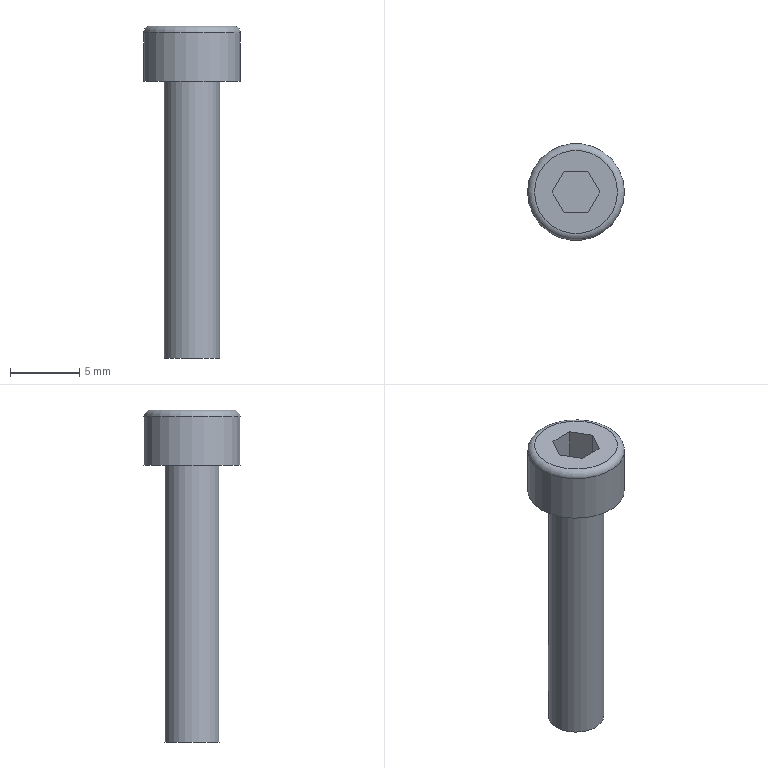Part | STEP file | Tube necking machine_id110_x_t | 1 solid | 13 faces | box 7 x 7 x 24 mm | volume 383.547 mm3 | plane 10 | cylinder 2 | torus 1 | commonest cylinder face diameters 4 x1 7 x1
STEP:
#1=CARTESIAN_POINT('',(0.,0.,0.));
#2=DIRECTION('',(0.,0.,1.));
#3=DIRECTION('',(1.,0.,0.));
#4=AXIS2_PLACEMENT_3D('',#1,#2,#3);
#5=CARTESIAN_POINT('',(-65.,62.5,245.1));
#6=VERTEX_POINT('',#5);
#7=CARTESIAN_POINT('',(-62.,62.5,245.1));
#8=DIRECTION('',(0.,0.,1.));
#9=DIRECTION('',(-1.,0.,0.));
#10=AXIS2_PLACEMENT_3D('',#7,#8,#9);
#11=CIRCLE('',#10,3.);
#12=CARTESIAN_POINT('',(-58.5,62.5,245.1));
#13=DIRECTION('',(0.,0.,-1.));
#14=DIRECTION('',(-1.,0.,0.));
#15=AXIS2_PLACEMENT_3D('',#12,#13,#14);
#16=PLANE('',#15);
#17=CARTESIAN_POINT('',(6.5,0.));
#18=CARTESIAN_POINT('',(6.5,-5.196));
#19=CARTESIAN_POINT('',(2.,-2.598));
#20=CARTESIAN_POINT('',(-2.5,0.));
#21=CARTESIAN_POINT('',(2.,2.598));
#22=CARTESIAN_POINT('',(6.5,5.196));
#23=CARTESIAN_POINT('',(6.5,0.));
#24=(BOUNDED_CURVE()B_SPLINE_CURVE(2,(#17,#18,#19,#20,#21,#22,#23),.UNSPECIFIED.,.T.,.F.)B_SPLINE_CURVE_WITH_KNOTS((1,2,2,2,2,1),(-2.094,0.,2.094,4.189,6.283,8.378),.UNSPECIFIED.)CURVE()GEOMETRIC_REPRESENTATION_ITEM()RATIONAL_B_SPLINE_CURVE((1.,0.5,1.,0.5,1.,0.5,1.))REPRESENTATION_ITEM(''));
#25=(GEOMETRIC_REPRESENTATION_CONTEXT(2)PARAMETRIC_REPRESENTATION_CONTEXT()REPRESENTATION_CONTEXT('',''));
#26=DEFINITIONAL_REPRESENTATION('',(#24),#25);
#27=PCURVE('',#16,#26);
#28=CARTESIAN_POINT('',(-62.,62.5,244.6));
#29=DIRECTION('',(0.,0.,-1.));
#30=DIRECTION('',(-1.,0.,0.));
#31=AXIS2_PLACEMENT_3D('',#28,#29,#30);
#32=TOROIDAL_SURFACE('',#31,3.,0.5);
#33=CARTESIAN_POINT('',(6.283,4.712));
#34=DIRECTION('',(-1.,0.));
#35=VECTOR('',#34,1.);
#36=LINE('',#33,#35);
#37=(GEOMETRIC_REPRESENTATION_CONTEXT(2)PARAMETRIC_REPRESENTATION_CONTEXT()REPRESENTATION_CONTEXT('',''));
#38=DEFINITIONAL_REPRESENTATION('',(#36),#37);
#39=PCURVE('',#32,#38);
#40=SURFACE_CURVE('',#11,(#27,#39),.PCURVE_S1.);
#41=EDGE_CURVE('',#6,#6,#40,.T.);
#42=ORIENTED_EDGE('',*,*,#41,.T.);
#43=EDGE_LOOP('',(#42));
#44=FACE_BOUND('',#43,.T.);
#45=CARTESIAN_POINT('',(-62.866,64.,245.1));
#46=VERTEX_POINT('',#45);
#47=CARTESIAN_POINT('',(-61.134,64.,245.1));
#48=VERTEX_POINT('',#47);
#49=CARTESIAN_POINT('',(-62.866,64.,245.1));
#50=DIRECTION('',(1.,0.,0.));
#51=VECTOR('',#50,1.);
#52=LINE('',#49,#51);
#53=CARTESIAN_POINT('',(4.366,1.5));
#54=DIRECTION('',(-1.,0.));
#55=VECTOR('',#54,1.);
#56=LINE('',#53,#55);
#57=(GEOMETRIC_REPRESENTATION_CONTEXT(2)PARAMETRIC_REPRESENTATION_CONTEXT()REPRESENTATION_CONTEXT('',''));
#58=DEFINITIONAL_REPRESENTATION('',(#56),#57);
#59=PCURVE('',#16,#58);
#60=CARTESIAN_POINT('',(-62.866,64.,242.46));
#61=DIRECTION('',(0.,-1.,0.));
#62=DIRECTION('',(1.,0.,0.));
#63=AXIS2_PLACEMENT_3D('',#60,#61,#62);
#64=PLANE('',#63);
#65=CARTESIAN_POINT('',(0.,2.64));
#66=DIRECTION('',(1.,0.));
#67=VECTOR('',#66,1.);
#68=LINE('',#65,#67);
#69=(GEOMETRIC_REPRESENTATION_CONTEXT(2)PARAMETRIC_REPRESENTATION_CONTEXT()REPRESENTATION_CONTEXT('',''));
#70=DEFINITIONAL_REPRESENTATION('',(#68),#69);
#71=PCURVE('',#64,#70);
#72=SURFACE_CURVE('',#52,(#59,#71),.PCURVE_S1.);
#73=EDGE_CURVE('',#46,#48,#72,.T.);
#74=ORIENTED_EDGE('',*,*,#73,.T.);
#75=CARTESIAN_POINT('',(-60.268,62.5,245.1));
#76=VERTEX_POINT('',#75);
#77=CARTESIAN_POINT('',(-61.134,64.,245.1));
#78=DIRECTION('',(0.5,-0.866,0.));
#79=VECTOR('',#78,1.);
#80=LINE('',#77,#79);
#81=CARTESIAN_POINT('',(2.634,1.5));
#82=DIRECTION('',(-0.5,-0.866));
#83=VECTOR('',#82,1.);
#84=LINE('',#81,#83);
#85=(GEOMETRIC_REPRESENTATION_CONTEXT(2)PARAMETRIC_REPRESENTATION_CONTEXT()REPRESENTATION_CONTEXT('',''));
#86=DEFINITIONAL_REPRESENTATION('',(#84),#85);
#87=PCURVE('',#16,#86);
#88=CARTESIAN_POINT('',(-61.134,64.,242.46));
#89=DIRECTION('',(-0.866,-0.5,0.));
#90=DIRECTION('',(0.5,-0.866,0.));
#91=AXIS2_PLACEMENT_3D('',#88,#89,#90);
#92=PLANE('',#91);
#93=CARTESIAN_POINT('',(0.,2.64));
#94=DIRECTION('',(1.,0.));
#95=VECTOR('',#94,1.);
#96=LINE('',#93,#95);
#97=(GEOMETRIC_REPRESENTATION_CONTEXT(2)PARAMETRIC_REPRESENTATION_CONTEXT()REPRESENTATION_CONTEXT('',''));
#98=DEFINITIONAL_REPRESENTATION('',(#96),#97);
#99=PCURVE('',#92,#98);
#100=SURFACE_CURVE('',#80,(#87,#99),.PCURVE_S1.);
#101=EDGE_CURVE('',#48,#76,#100,.T.);
#102=ORIENTED_EDGE('',*,*,#101,.T.);
#103=CARTESIAN_POINT('',(-61.134,61.,245.1));
#104=VERTEX_POINT('',#103);
#105=CARTESIAN_POINT('',(-60.268,62.5,245.1));
#106=DIRECTION('',(-0.5,-0.866,0.));
#107=VECTOR('',#106,1.);
#108=LINE('',#105,#107);
#109=CARTESIAN_POINT('',(1.768,0.));
#110=DIRECTION('',(0.5,-0.866));
#111=VECTOR('',#110,1.);
#112=LINE('',#109,#111);
#113=(GEOMETRIC_REPRESENTATION_CONTEXT(2)PARAMETRIC_REPRESENTATION_CONTEXT()REPRESENTATION_CONTEXT('',''));
#114=DEFINITIONAL_REPRESENTATION('',(#112),#113);
#115=PCURVE('',#16,#114);
#116=CARTESIAN_POINT('',(-60.268,62.5,242.46));
#117=DIRECTION('',(-0.866,0.5,0.));
#118=DIRECTION('',(-0.5,-0.866,0.));
#119=AXIS2_PLACEMENT_3D('',#116,#117,#118);
#120=PLANE('',#119);
#121=CARTESIAN_POINT('',(0.,2.64));
#122=DIRECTION('',(1.,0.));
#123=VECTOR('',#122,1.);
#124=LINE('',#121,#123);
#125=(GEOMETRIC_REPRESENTATION_CONTEXT(2)PARAMETRIC_REPRESENTATION_CONTEXT()REPRESENTATION_CONTEXT('',''));
#126=DEFINITIONAL_REPRESENTATION('',(#124),#125);
#127=PCURVE('',#120,#126);
#128=SURFACE_CURVE('',#108,(#115,#127),.PCURVE_S1.);
#129=EDGE_CURVE('',#76,#104,#128,.T.);
#130=ORIENTED_EDGE('',*,*,#129,.T.);
#131=CARTESIAN_POINT('',(-62.866,61.,245.1));
#132=VERTEX_POINT('',#131);
#133=CARTESIAN_POINT('',(-61.134,61.,245.1));
#134=DIRECTION('',(-1.,0.,0.));
#135=VECTOR('',#134,1.);
#136=LINE('',#133,#135);
#137=CARTESIAN_POINT('',(2.634,-1.5));
#138=DIRECTION('',(1.,0.));
#139=VECTOR('',#138,1.);
#140=LINE('',#137,#139);
#141=(GEOMETRIC_REPRESENTATION_CONTEXT(2)PARAMETRIC_REPRESENTATION_CONTEXT()REPRESENTATION_CONTEXT('',''));
#142=DEFINITIONAL_REPRESENTATION('',(#140),#141);
#143=PCURVE('',#16,#142);
#144=CARTESIAN_POINT('',(-61.134,61.,242.46));
#145=DIRECTION('',(0.,1.,0.));
#146=DIRECTION('',(-1.,0.,0.));
#147=AXIS2_PLACEMENT_3D('',#144,#145,#146);
#148=PLANE('',#147);
#149=CARTESIAN_POINT('',(0.,2.64));
#150=DIRECTION('',(1.,0.));
#151=VECTOR('',#150,1.);
#152=LINE('',#149,#151);
#153=(GEOMETRIC_REPRESENTATION_CONTEXT(2)PARAMETRIC_REPRESENTATION_CONTEXT()REPRESENTATION_CONTEXT('',''));
#154=DEFINITIONAL_REPRESENTATION('',(#152),#153);
#155=PCURVE('',#148,#154);
#156=SURFACE_CURVE('',#136,(#143,#155),.PCURVE_S1.);
#157=EDGE_CURVE('',#104,#132,#156,.T.);
#158=ORIENTED_EDGE('',*,*,#157,.T.);
#159=CARTESIAN_POINT('',(-63.732,62.5,245.1));
#160=VERTEX_POINT('',#159);
#161=CARTESIAN_POINT('',(-62.866,61.,245.1));
#162=DIRECTION('',(-0.5,0.866,0.));
#163=VECTOR('',#162,1.);
#164=LINE('',#161,#163);
#165=CARTESIAN_POINT('',(4.366,-1.5));
#166=DIRECTION('',(0.5,0.866));
#167=VECTOR('',#166,1.);
#168=LINE('',#165,#167);
#169=(GEOMETRIC_REPRESENTATION_CONTEXT(2)PARAMETRIC_REPRESENTATION_CONTEXT()REPRESENTATION_CONTEXT('',''));
#170=DEFINITIONAL_REPRESENTATION('',(#168),#169);
#171=PCURVE('',#16,#170);
#172=CARTESIAN_POINT('',(-62.866,61.,242.46));
#173=DIRECTION('',(0.866,0.5,0.));
#174=DIRECTION('',(-0.5,0.866,0.));
#175=AXIS2_PLACEMENT_3D('',#172,#173,#174);
#176=PLANE('',#175);
#177=CARTESIAN_POINT('',(0.,2.64));
#178=DIRECTION('',(1.,0.));
#179=VECTOR('',#178,1.);
#180=LINE('',#177,#179);
#181=(GEOMETRIC_REPRESENTATION_CONTEXT(2)PARAMETRIC_REPRESENTATION_CONTEXT()REPRESENTATION_CONTEXT('',''));
#182=DEFINITIONAL_REPRESENTATION('',(#180),#181);
#183=PCURVE('',#176,#182);
#184=SURFACE_CURVE('',#164,(#171,#183),.PCURVE_S1.);
#185=EDGE_CURVE('',#132,#160,#184,.T.);
#186=ORIENTED_EDGE('',*,*,#185,.T.);
#187=CARTESIAN_POINT('',(-63.732,62.5,245.1));
#188=DIRECTION('',(0.5,0.866,0.));
#189=VECTOR('',#188,1.);
#190=LINE('',#187,#189);
#191=CARTESIAN_POINT('',(5.232,0.));
#192=DIRECTION('',(-0.5,0.866));
#193=VECTOR('',#192,1.);
#194=LINE('',#191,#193);
#195=(GEOMETRIC_REPRESENTATION_CONTEXT(2)PARAMETRIC_REPRESENTATION_CONTEXT()REPRESENTATION_CONTEXT('',''));
#196=DEFINITIONAL_REPRESENTATION('',(#194),#195);
#197=PCURVE('',#16,#196);
#198=CARTESIAN_POINT('',(-63.732,62.5,242.46));
#199=DIRECTION('',(0.866,-0.5,0.));
#200=DIRECTION('',(0.5,0.866,0.));
#201=AXIS2_PLACEMENT_3D('',#198,#199,#200);
#202=PLANE('',#201);
#203=CARTESIAN_POINT('',(0.,2.64));
#204=DIRECTION('',(1.,0.));
#205=VECTOR('',#204,1.);
#206=LINE('',#203,#205);
#207=(GEOMETRIC_REPRESENTATION_CONTEXT(2)PARAMETRIC_REPRESENTATION_CONTEXT()REPRESENTATION_CONTEXT('',''));
#208=DEFINITIONAL_REPRESENTATION('',(#206),#207);
#209=PCURVE('',#202,#208);
#210=SURFACE_CURVE('',#190,(#197,#209),.PCURVE_S1.);
#211=EDGE_CURVE('',#160,#46,#210,.T.);
#212=ORIENTED_EDGE('',*,*,#211,.T.);
#213=EDGE_LOOP('',(#74,#102,#130,#158,#186,#212));
#214=FACE_BOUND('',#213,.T.);
#215=ADVANCED_FACE('',(#44,#214),#16,.F.);
#216=CARTESIAN_POINT('',(-65.5,62.5,244.6));
#217=VERTEX_POINT('',#216);
#218=CARTESIAN_POINT('',(-58.5,62.5,244.6));
#219=VERTEX_POINT('',#218);
#220=CARTESIAN_POINT('',(-62.,62.5,244.6));
#221=DIRECTION('',(0.,0.,-1.));
#222=DIRECTION('',(-1.,0.,0.));
#223=AXIS2_PLACEMENT_3D('',#220,#221,#222);
#224=CIRCLE('',#223,3.5);
#225=CARTESIAN_POINT('',(-62.,62.5,242.2));
#226=DIRECTION('',(0.,0.,1.));
#227=DIRECTION('',(1.,0.,0.));
#228=AXIS2_PLACEMENT_3D('',#225,#226,#227);
#229=CYLINDRICAL_SURFACE('',#228,3.5);
#230=CARTESIAN_POINT('',(3.142,2.4));
#231=DIRECTION('',(-1.,0.));
#232=VECTOR('',#231,1.);
#233=LINE('',#230,#232);
#234=(GEOMETRIC_REPRESENTATION_CONTEXT(2)PARAMETRIC_REPRESENTATION_CONTEXT()REPRESENTATION_CONTEXT('',''));
#235=DEFINITIONAL_REPRESENTATION('',(#233),#234);
#236=PCURVE('',#229,#235);
#237=CARTESIAN_POINT('',(0.,6.283));
#238=DIRECTION('',(1.,0.));
#239=VECTOR('',#238,1.);
#240=LINE('',#237,#239);
#241=(GEOMETRIC_REPRESENTATION_CONTEXT(2)PARAMETRIC_REPRESENTATION_CONTEXT()REPRESENTATION_CONTEXT('',''));
#242=DEFINITIONAL_REPRESENTATION('',(#240),#241);
#243=PCURVE('',#32,#242);
#244=SURFACE_CURVE('',#224,(#236,#243),.PCURVE_S1.);
#245=EDGE_CURVE('',#217,#219,#244,.T.);
#246=ORIENTED_EDGE('',*,*,#245,.T.);
#247=CARTESIAN_POINT('',(-58.5,62.5,241.1));
#248=VERTEX_POINT('',#247);
#249=CARTESIAN_POINT('',(-58.5,62.5,241.1));
#250=CARTESIAN_POINT('',(-58.5,62.5,244.6));
#251=B_SPLINE_CURVE_WITH_KNOTS('',1,(#249,#250),.UNSPECIFIED.,.F.,.F.,(2,2),(-1.1,2.4),.PIECEWISE_BEZIER_KNOTS.);
#252=CARTESIAN_POINT('',(0.,0.));
#253=DIRECTION('',(0.,1.));
#254=VECTOR('',#253,1.);
#255=LINE('',#252,#254);
#256=(GEOMETRIC_REPRESENTATION_CONTEXT(2)PARAMETRIC_REPRESENTATION_CONTEXT()REPRESENTATION_CONTEXT('',''));
#257=DEFINITIONAL_REPRESENTATION('',(#255),#256);
#258=PCURVE('',#229,#257);
#259=CARTESIAN_POINT('',(6.283,0.));
#260=DIRECTION('',(0.,1.));
#261=VECTOR('',#260,1.);
#262=LINE('',#259,#261);
#263=(GEOMETRIC_REPRESENTATION_CONTEXT(2)PARAMETRIC_REPRESENTATION_CONTEXT()REPRESENTATION_CONTEXT('',''));
#264=DEFINITIONAL_REPRESENTATION('',(#262),#263);
#265=PCURVE('',#229,#264);
#266=SEAM_CURVE('',#251,(#258,#265),.PCURVE_S1.);
#267=EDGE_CURVE('',#248,#219,#266,.T.);
#268=ORIENTED_EDGE('',*,*,#267,.F.);
#269=CARTESIAN_POINT('',(-62.,62.5,241.1));
#270=DIRECTION('',(0.,0.,1.));
#271=DIRECTION('',(1.,0.,0.));
#272=AXIS2_PLACEMENT_3D('',#269,#270,#271);
#273=CIRCLE('',#272,3.5);
#274=CARTESIAN_POINT('',(0.,-1.1));
#275=DIRECTION('',(1.,0.));
#276=VECTOR('',#275,1.);
#277=LINE('',#274,#276);
#278=(GEOMETRIC_REPRESENTATION_CONTEXT(2)PARAMETRIC_REPRESENTATION_CONTEXT()REPRESENTATION_CONTEXT('',''));
#279=DEFINITIONAL_REPRESENTATION('',(#277),#278);
#280=PCURVE('',#229,#279);
#281=CARTESIAN_POINT('',(-60.,62.5,241.1));
#282=DIRECTION('',(0.,0.,1.));
#283=DIRECTION('',(1.,0.,0.));
#284=AXIS2_PLACEMENT_3D('',#281,#282,#283);
#285=PLANE('',#284);
#286=CARTESIAN_POINT('',(-2.,0.));
#287=DIRECTION('',(1.,0.));
#288=AXIS2_PLACEMENT_2D('',#286,#287);
#289=CIRCLE('',#288,3.5);
#290=(GEOMETRIC_REPRESENTATION_CONTEXT(2)PARAMETRIC_REPRESENTATION_CONTEXT()REPRESENTATION_CONTEXT('',''));
#291=DEFINITIONAL_REPRESENTATION('',(#289),#290);
#292=PCURVE('',#285,#291);
#293=SURFACE_CURVE('',#273,(#280,#292),.PCURVE_S1.);
#294=EDGE_CURVE('',#248,#248,#293,.T.);
#295=ORIENTED_EDGE('',*,*,#294,.T.);
#296=ORIENTED_EDGE('',*,*,#267,.T.);
#297=CARTESIAN_POINT('',(-62.,62.5,244.6));
#298=DIRECTION('',(0.,0.,-1.));
#299=DIRECTION('',(-1.,0.,0.));
#300=AXIS2_PLACEMENT_3D('',#297,#298,#299);
#301=CIRCLE('',#300,3.5);
#302=CARTESIAN_POINT('',(9.425,2.4));
#303=DIRECTION('',(-1.,0.));
#304=VECTOR('',#303,1.);
#305=LINE('',#302,#304);
#306=(GEOMETRIC_REPRESENTATION_CONTEXT(2)PARAMETRIC_REPRESENTATION_CONTEXT()REPRESENTATION_CONTEXT('',''));
#307=DEFINITIONAL_REPRESENTATION('',(#305),#306);
#308=PCURVE('',#229,#307);
#309=CARTESIAN_POINT('',(0.,6.283));
#310=DIRECTION('',(1.,0.));
#311=VECTOR('',#310,1.);
#312=LINE('',#309,#311);
#313=(GEOMETRIC_REPRESENTATION_CONTEXT(2)PARAMETRIC_REPRESENTATION_CONTEXT()REPRESENTATION_CONTEXT('',''));
#314=DEFINITIONAL_REPRESENTATION('',(#312),#313);
#315=PCURVE('',#32,#314);
#316=SURFACE_CURVE('',#301,(#308,#315),.PCURVE_S1.);
#317=EDGE_CURVE('',#219,#217,#316,.T.);
#318=ORIENTED_EDGE('',*,*,#317,.T.);
#319=EDGE_LOOP('',(#246,#268,#295,#296,#318));
#320=FACE_BOUND('',#319,.T.);
#321=ADVANCED_FACE('',(#320),#229,.T.);
#322=ORIENTED_EDGE('',*,*,#294,.F.);
#323=EDGE_LOOP('',(#322));
#324=FACE_BOUND('',#323,.T.);
#325=CARTESIAN_POINT('',(-60.,62.5,241.1));
#326=VERTEX_POINT('',#325);
#327=CARTESIAN_POINT('',(-62.,62.5,241.1));
#328=DIRECTION('',(0.,0.,1.));
#329=DIRECTION('',(1.,0.,0.));
#330=AXIS2_PLACEMENT_3D('',#327,#328,#329);
#331=CIRCLE('',#330,2.);
#332=CARTESIAN_POINT('',(-2.,0.));
#333=DIRECTION('',(1.,0.));
#334=AXIS2_PLACEMENT_2D('',#332,#333);
#335=CIRCLE('',#334,2.);
#336=(GEOMETRIC_REPRESENTATION_CONTEXT(2)PARAMETRIC_REPRESENTATION_CONTEXT()REPRESENTATION_CONTEXT('',''));
#337=DEFINITIONAL_REPRESENTATION('',(#335),#336);
#338=PCURVE('',#285,#337);
#339=CARTESIAN_POINT('',(-62.,62.5,242.2));
#340=DIRECTION('',(0.,0.,1.));
#341=DIRECTION('',(1.,0.,0.));
#342=AXIS2_PLACEMENT_3D('',#339,#340,#341);
#343=CYLINDRICAL_SURFACE('',#342,2.);
#344=CARTESIAN_POINT('',(0.,-1.1));
#345=DIRECTION('',(1.,0.));
#346=VECTOR('',#345,1.);
#347=LINE('',#344,#346);
#348=(GEOMETRIC_REPRESENTATION_CONTEXT(2)PARAMETRIC_REPRESENTATION_CONTEXT()REPRESENTATION_CONTEXT('',''));
#349=DEFINITIONAL_REPRESENTATION('',(#347),#348);
#350=PCURVE('',#343,#349);
#351=SURFACE_CURVE('',#331,(#338,#350),.PCURVE_S1.);
#352=EDGE_CURVE('',#326,#326,#351,.T.);
#353=ORIENTED_EDGE('',*,*,#352,.T.);
#354=EDGE_LOOP('',(#353));
#355=FACE_BOUND('',#354,.T.);
#356=ADVANCED_FACE('',(#324,#355),#285,.F.);
#357=ORIENTED_EDGE('',*,*,#352,.F.);
#358=CARTESIAN_POINT('',(-60.,62.5,221.1));
#359=VERTEX_POINT('',#358);
#360=CARTESIAN_POINT('',(-60.,62.5,221.1));
#361=CARTESIAN_POINT('',(-60.,62.5,241.1));
#362=B_SPLINE_CURVE_WITH_KNOTS('',1,(#360,#361),.UNSPECIFIED.,.F.,.F.,(2,2),(-21.1,-1.1),.PIECEWISE_BEZIER_KNOTS.);
#363=CARTESIAN_POINT('',(0.,0.));
#364=DIRECTION('',(0.,1.));
#365=VECTOR('',#364,1.);
#366=LINE('',#363,#365);
#367=(GEOMETRIC_REPRESENTATION_CONTEXT(2)PARAMETRIC_REPRESENTATION_CONTEXT()REPRESENTATION_CONTEXT('',''));
#368=DEFINITIONAL_REPRESENTATION('',(#366),#367);
#369=PCURVE('',#343,#368);
#370=CARTESIAN_POINT('',(6.283,0.));
#371=DIRECTION('',(0.,1.));
#372=VECTOR('',#371,1.);
#373=LINE('',#370,#372);
#374=(GEOMETRIC_REPRESENTATION_CONTEXT(2)PARAMETRIC_REPRESENTATION_CONTEXT()REPRESENTATION_CONTEXT('',''));
#375=DEFINITIONAL_REPRESENTATION('',(#373),#374);
#376=PCURVE('',#343,#375);
#377=SEAM_CURVE('',#362,(#369,#376),.PCURVE_S1.);
#378=EDGE_CURVE('',#359,#326,#377,.T.);
#379=ORIENTED_EDGE('',*,*,#378,.F.);
#380=CARTESIAN_POINT('',(-62.,62.5,221.1));
#381=DIRECTION('',(0.,0.,1.));
#382=DIRECTION('',(1.,0.,0.));
#383=AXIS2_PLACEMENT_3D('',#380,#381,#382);
#384=CIRCLE('',#383,2.);
#385=CARTESIAN_POINT('',(0.,-21.1));
#386=DIRECTION('',(1.,0.));
#387=VECTOR('',#386,1.);
#388=LINE('',#385,#387);
#389=(GEOMETRIC_REPRESENTATION_CONTEXT(2)PARAMETRIC_REPRESENTATION_CONTEXT()REPRESENTATION_CONTEXT('',''));
#390=DEFINITIONAL_REPRESENTATION('',(#388),#389);
#391=PCURVE('',#343,#390);
#392=CARTESIAN_POINT('',(-62.,62.5,221.1));
#393=DIRECTION('',(0.,0.,1.));
#394=DIRECTION('',(1.,0.,0.));
#395=AXIS2_PLACEMENT_3D('',#392,#393,#394);
#396=PLANE('',#395);
#397=CARTESIAN_POINT('',(0.,0.));
#398=DIRECTION('',(1.,0.));
#399=AXIS2_PLACEMENT_2D('',#397,#398);
#400=CIRCLE('',#399,2.);
#401=(GEOMETRIC_REPRESENTATION_CONTEXT(2)PARAMETRIC_REPRESENTATION_CONTEXT()REPRESENTATION_CONTEXT('',''));
#402=DEFINITIONAL_REPRESENTATION('',(#400),#401);
#403=PCURVE('',#396,#402);
#404=SURFACE_CURVE('',#384,(#391,#403),.PCURVE_S1.);
#405=EDGE_CURVE('',#359,#359,#404,.T.);
#406=ORIENTED_EDGE('',*,*,#405,.T.);
#407=ORIENTED_EDGE('',*,*,#378,.T.);
#408=EDGE_LOOP('',(#357,#379,#406,#407));
#409=FACE_BOUND('',#408,.T.);
#410=ADVANCED_FACE('',(#409),#343,.T.);
#411=ORIENTED_EDGE('',*,*,#405,.F.);
#412=EDGE_LOOP('',(#411));
#413=FACE_BOUND('',#412,.T.);
#414=ADVANCED_FACE('',(#413),#396,.F.);
#415=ORIENTED_EDGE('',*,*,#73,.F.);
#416=CARTESIAN_POINT('',(-62.866,64.,242.46));
#417=VERTEX_POINT('',#416);
#418=CARTESIAN_POINT('',(-62.866,64.,242.46));
#419=DIRECTION('',(0.,0.,-1.));
#420=VECTOR('',#419,1.);
#421=LINE('',#418,#420);
#422=CARTESIAN_POINT('',(0.,0.));
#423=DIRECTION('',(0.,-1.));
#424=VECTOR('',#423,1.);
#425=LINE('',#422,#424);
#426=(GEOMETRIC_REPRESENTATION_CONTEXT(2)PARAMETRIC_REPRESENTATION_CONTEXT()REPRESENTATION_CONTEXT('',''));
#427=DEFINITIONAL_REPRESENTATION('',(#425),#426);
#428=PCURVE('',#64,#427);
#429=CARTESIAN_POINT('',(1.732,0.));
#430=DIRECTION('',(0.,-1.));
#431=VECTOR('',#430,1.);
#432=LINE('',#429,#431);
#433=(GEOMETRIC_REPRESENTATION_CONTEXT(2)PARAMETRIC_REPRESENTATION_CONTEXT()REPRESENTATION_CONTEXT('',''));
#434=DEFINITIONAL_REPRESENTATION('',(#432),#433);
#435=PCURVE('',#202,#434);
#436=SURFACE_CURVE('',#421,(#428,#435),.PCURVE_S1.);
#437=EDGE_CURVE('',#46,#417,#436,.T.);
#438=ORIENTED_EDGE('',*,*,#437,.T.);
#439=CARTESIAN_POINT('',(-61.134,64.,242.46));
#440=VERTEX_POINT('',#439);
#441=CARTESIAN_POINT('',(-62.866,64.,242.46));
#442=DIRECTION('',(-1.,0.,0.));
#443=VECTOR('',#442,1.);
#444=LINE('',#441,#443);
#445=CARTESIAN_POINT('',(0.,0.));
#446=DIRECTION('',(-1.,0.));
#447=VECTOR('',#446,1.);
#448=LINE('',#445,#447);
#449=(GEOMETRIC_REPRESENTATION_CONTEXT(2)PARAMETRIC_REPRESENTATION_CONTEXT()REPRESENTATION_CONTEXT('',''));
#450=DEFINITIONAL_REPRESENTATION('',(#448),#449);
#451=PCURVE('',#64,#450);
#452=CARTESIAN_POINT('',(-62.,62.5,242.46));
#453=DIRECTION('',(0.,0.,-1.));
#454=DIRECTION('',(-1.,0.,0.));
#455=AXIS2_PLACEMENT_3D('',#452,#453,#454);
#456=PLANE('',#455);
#457=CARTESIAN_POINT('',(0.866,1.5));
#458=DIRECTION('',(1.,0.));
#459=VECTOR('',#458,1.);
#460=LINE('',#457,#459);
#461=(GEOMETRIC_REPRESENTATION_CONTEXT(2)PARAMETRIC_REPRESENTATION_CONTEXT()REPRESENTATION_CONTEXT('',''));
#462=DEFINITIONAL_REPRESENTATION('',(#460),#461);
#463=PCURVE('',#456,#462);
#464=SURFACE_CURVE('',#444,(#451,#463),.PCURVE_S1.);
#465=EDGE_CURVE('',#440,#417,#464,.T.);
#466=ORIENTED_EDGE('',*,*,#465,.F.);
#467=CARTESIAN_POINT('',(-61.134,64.,242.46));
#468=DIRECTION('',(0.,0.,-1.));
#469=VECTOR('',#468,1.);
#470=LINE('',#467,#469);
#471=CARTESIAN_POINT('',(1.732,0.));
#472=DIRECTION('',(0.,-1.));
#473=VECTOR('',#472,1.);
#474=LINE('',#471,#473);
#475=(GEOMETRIC_REPRESENTATION_CONTEXT(2)PARAMETRIC_REPRESENTATION_CONTEXT()REPRESENTATION_CONTEXT('',''));
#476=DEFINITIONAL_REPRESENTATION('',(#474),#475);
#477=PCURVE('',#64,#476);
#478=CARTESIAN_POINT('',(0.,0.));
#479=DIRECTION('',(0.,-1.));
#480=VECTOR('',#479,1.);
#481=LINE('',#478,#480);
#482=(GEOMETRIC_REPRESENTATION_CONTEXT(2)PARAMETRIC_REPRESENTATION_CONTEXT()REPRESENTATION_CONTEXT('',''));
#483=DEFINITIONAL_REPRESENTATION('',(#481),#482);
#484=PCURVE('',#92,#483);
#485=SURFACE_CURVE('',#470,(#477,#484),.PCURVE_S1.);
#486=EDGE_CURVE('',#48,#440,#485,.T.);
#487=ORIENTED_EDGE('',*,*,#486,.F.);
#488=EDGE_LOOP('',(#415,#438,#466,#487));
#489=FACE_BOUND('',#488,.T.);
#490=ADVANCED_FACE('',(#489),#64,.T.);
#491=ORIENTED_EDGE('',*,*,#101,.F.);
#492=ORIENTED_EDGE('',*,*,#486,.T.);
#493=CARTESIAN_POINT('',(-60.268,62.5,242.46));
#494=VERTEX_POINT('',#493);
#495=CARTESIAN_POINT('',(-61.134,64.,242.46));
#496=DIRECTION('',(-0.5,0.866,0.));
#497=VECTOR('',#496,1.);
#498=LINE('',#495,#497);
#499=CARTESIAN_POINT('',(0.,0.));
#500=DIRECTION('',(-1.,0.));
#501=VECTOR('',#500,1.);
#502=LINE('',#499,#501);
#503=(GEOMETRIC_REPRESENTATION_CONTEXT(2)PARAMETRIC_REPRESENTATION_CONTEXT()REPRESENTATION_CONTEXT('',''));
#504=DEFINITIONAL_REPRESENTATION('',(#502),#503);
#505=PCURVE('',#92,#504);
#506=CARTESIAN_POINT('',(-0.866,1.5));
#507=DIRECTION('',(0.5,0.866));
#508=VECTOR('',#507,1.);
#509=LINE('',#506,#508);
#510=(GEOMETRIC_REPRESENTATION_CONTEXT(2)PARAMETRIC_REPRESENTATION_CONTEXT()REPRESENTATION_CONTEXT('',''));
#511=DEFINITIONAL_REPRESENTATION('',(#509),#510);
#512=PCURVE('',#456,#511);
#513=SURFACE_CURVE('',#498,(#505,#512),.PCURVE_S1.);
#514=EDGE_CURVE('',#494,#440,#513,.T.);
#515=ORIENTED_EDGE('',*,*,#514,.F.);
#516=CARTESIAN_POINT('',(-60.268,62.5,242.46));
#517=DIRECTION('',(0.,0.,-1.));
#518=VECTOR('',#517,1.);
#519=LINE('',#516,#518);
#520=CARTESIAN_POINT('',(1.732,0.));
#521=DIRECTION('',(0.,-1.));
#522=VECTOR('',#521,1.);
#523=LINE('',#520,#522);
#524=(GEOMETRIC_REPRESENTATION_CONTEXT(2)PARAMETRIC_REPRESENTATION_CONTEXT()REPRESENTATION_CONTEXT('',''));
#525=DEFINITIONAL_REPRESENTATION('',(#523),#524);
#526=PCURVE('',#92,#525);
#527=CARTESIAN_POINT('',(0.,0.));
#528=DIRECTION('',(0.,-1.));
#529=VECTOR('',#528,1.);
#530=LINE('',#527,#529);
#531=(GEOMETRIC_REPRESENTATION_CONTEXT(2)PARAMETRIC_REPRESENTATION_CONTEXT()REPRESENTATION_CONTEXT('',''));
#532=DEFINITIONAL_REPRESENTATION('',(#530),#531);
#533=PCURVE('',#120,#532);
#534=SURFACE_CURVE('',#519,(#526,#533),.PCURVE_S1.);
#535=EDGE_CURVE('',#76,#494,#534,.T.);
#536=ORIENTED_EDGE('',*,*,#535,.F.);
#537=EDGE_LOOP('',(#491,#492,#515,#536));
#538=FACE_BOUND('',#537,.T.);
#539=ADVANCED_FACE('',(#538),#92,.T.);
#540=ORIENTED_EDGE('',*,*,#129,.F.);
#541=ORIENTED_EDGE('',*,*,#535,.T.);
#542=CARTESIAN_POINT('',(-61.134,61.,242.46));
#543=VERTEX_POINT('',#542);
#544=CARTESIAN_POINT('',(-60.268,62.5,242.46));
#545=DIRECTION('',(0.5,0.866,0.));
#546=VECTOR('',#545,1.);
#547=LINE('',#544,#546);
#548=CARTESIAN_POINT('',(0.,0.));
#549=DIRECTION('',(-1.,0.));
#550=VECTOR('',#549,1.);
#551=LINE('',#548,#550);
#552=(GEOMETRIC_REPRESENTATION_CONTEXT(2)PARAMETRIC_REPRESENTATION_CONTEXT()REPRESENTATION_CONTEXT('',''));
#553=DEFINITIONAL_REPRESENTATION('',(#551),#552);
#554=PCURVE('',#120,#553);
#555=CARTESIAN_POINT('',(-1.732,0.));
#556=DIRECTION('',(-0.5,0.866));
#557=VECTOR('',#556,1.);
#558=LINE('',#555,#557);
#559=(GEOMETRIC_REPRESENTATION_CONTEXT(2)PARAMETRIC_REPRESENTATION_CONTEXT()REPRESENTATION_CONTEXT('',''));
#560=DEFINITIONAL_REPRESENTATION('',(#558),#559);
#561=PCURVE('',#456,#560);
#562=SURFACE_CURVE('',#547,(#554,#561),.PCURVE_S1.);
#563=EDGE_CURVE('',#543,#494,#562,.T.);
#564=ORIENTED_EDGE('',*,*,#563,.F.);
#565=CARTESIAN_POINT('',(-61.134,61.,242.46));
#566=DIRECTION('',(0.,0.,-1.));
#567=VECTOR('',#566,1.);
#568=LINE('',#565,#567);
#569=CARTESIAN_POINT('',(1.732,0.));
#570=DIRECTION('',(0.,-1.));
#571=VECTOR('',#570,1.);
#572=LINE('',#569,#571);
#573=(GEOMETRIC_REPRESENTATION_CONTEXT(2)PARAMETRIC_REPRESENTATION_CONTEXT()REPRESENTATION_CONTEXT('',''));
#574=DEFINITIONAL_REPRESENTATION('',(#572),#573);
#575=PCURVE('',#120,#574);
#576=CARTESIAN_POINT('',(0.,0.));
#577=DIRECTION('',(0.,-1.));
#578=VECTOR('',#577,1.);
#579=LINE('',#576,#578);
#580=(GEOMETRIC_REPRESENTATION_CONTEXT(2)PARAMETRIC_REPRESENTATION_CONTEXT()REPRESENTATION_CONTEXT('',''));
#581=DEFINITIONAL_REPRESENTATION('',(#579),#580);
#582=PCURVE('',#148,#581);
#583=SURFACE_CURVE('',#568,(#575,#582),.PCURVE_S1.);
#584=EDGE_CURVE('',#104,#543,#583,.T.);
#585=ORIENTED_EDGE('',*,*,#584,.F.);
#586=EDGE_LOOP('',(#540,#541,#564,#585));
#587=FACE_BOUND('',#586,.T.);
#588=ADVANCED_FACE('',(#587),#120,.T.);
#589=ORIENTED_EDGE('',*,*,#157,.F.);
#590=ORIENTED_EDGE('',*,*,#584,.T.);
#591=CARTESIAN_POINT('',(-62.866,61.,242.46));
#592=VERTEX_POINT('',#591);
#593=CARTESIAN_POINT('',(-61.134,61.,242.46));
#594=DIRECTION('',(1.,0.,0.));
#595=VECTOR('',#594,1.);
#596=LINE('',#593,#595);
#597=CARTESIAN_POINT('',(0.,0.));
#598=DIRECTION('',(-1.,0.));
#599=VECTOR('',#598,1.);
#600=LINE('',#597,#599);
#601=(GEOMETRIC_REPRESENTATION_CONTEXT(2)PARAMETRIC_REPRESENTATION_CONTEXT()REPRESENTATION_CONTEXT('',''));
#602=DEFINITIONAL_REPRESENTATION('',(#600),#601);
#603=PCURVE('',#148,#602);
#604=CARTESIAN_POINT('',(-0.866,-1.5));
#605=DIRECTION('',(-1.,0.));
#606=VECTOR('',#605,1.);
#607=LINE('',#604,#606);
#608=(GEOMETRIC_REPRESENTATION_CONTEXT(2)PARAMETRIC_REPRESENTATION_CONTEXT()REPRESENTATION_CONTEXT('',''));
#609=DEFINITIONAL_REPRESENTATION('',(#607),#608);
#610=PCURVE('',#456,#609);
#611=SURFACE_CURVE('',#596,(#603,#610),.PCURVE_S1.);
#612=EDGE_CURVE('',#592,#543,#611,.T.);
#613=ORIENTED_EDGE('',*,*,#612,.F.);
#614=CARTESIAN_POINT('',(-62.866,61.,242.46));
#615=DIRECTION('',(0.,0.,-1.));
#616=VECTOR('',#615,1.);
#617=LINE('',#614,#616);
#618=CARTESIAN_POINT('',(1.732,0.));
#619=DIRECTION('',(0.,-1.));
#620=VECTOR('',#619,1.);
#621=LINE('',#618,#620);
#622=(GEOMETRIC_REPRESENTATION_CONTEXT(2)PARAMETRIC_REPRESENTATION_CONTEXT()REPRESENTATION_CONTEXT('',''));
#623=DEFINITIONAL_REPRESENTATION('',(#621),#622);
#624=PCURVE('',#148,#623);
#625=CARTESIAN_POINT('',(0.,0.));
#626=DIRECTION('',(0.,-1.));
#627=VECTOR('',#626,1.);
#628=LINE('',#625,#627);
#629=(GEOMETRIC_REPRESENTATION_CONTEXT(2)PARAMETRIC_REPRESENTATION_CONTEXT()REPRESENTATION_CONTEXT('',''));
#630=DEFINITIONAL_REPRESENTATION('',(#628),#629);
#631=PCURVE('',#176,#630);
#632=SURFACE_CURVE('',#617,(#624,#631),.PCURVE_S1.);
#633=EDGE_CURVE('',#132,#592,#632,.T.);
#634=ORIENTED_EDGE('',*,*,#633,.F.);
#635=EDGE_LOOP('',(#589,#590,#613,#634));
#636=FACE_BOUND('',#635,.T.);
#637=ADVANCED_FACE('',(#636),#148,.T.);
#638=ORIENTED_EDGE('',*,*,#185,.F.);
#639=ORIENTED_EDGE('',*,*,#633,.T.);
#640=CARTESIAN_POINT('',(-63.732,62.5,242.46));
#641=VERTEX_POINT('',#640);
#642=CARTESIAN_POINT('',(-62.866,61.,242.46));
#643=DIRECTION('',(0.5,-0.866,0.));
#644=VECTOR('',#643,1.);
#645=LINE('',#642,#644);
#646=CARTESIAN_POINT('',(0.,0.));
#647=DIRECTION('',(-1.,0.));
#648=VECTOR('',#647,1.);
#649=LINE('',#646,#648);
#650=(GEOMETRIC_REPRESENTATION_CONTEXT(2)PARAMETRIC_REPRESENTATION_CONTEXT()REPRESENTATION_CONTEXT('',''));
#651=DEFINITIONAL_REPRESENTATION('',(#649),#650);
#652=PCURVE('',#176,#651);
#653=CARTESIAN_POINT('',(0.866,-1.5));
#654=DIRECTION('',(-0.5,-0.866));
#655=VECTOR('',#654,1.);
#656=LINE('',#653,#655);
#657=(GEOMETRIC_REPRESENTATION_CONTEXT(2)PARAMETRIC_REPRESENTATION_CONTEXT()REPRESENTATION_CONTEXT('',''));
#658=DEFINITIONAL_REPRESENTATION('',(#656),#657);
#659=PCURVE('',#456,#658);
#660=SURFACE_CURVE('',#645,(#652,#659),.PCURVE_S1.);
#661=EDGE_CURVE('',#641,#592,#660,.T.);
#662=ORIENTED_EDGE('',*,*,#661,.F.);
#663=CARTESIAN_POINT('',(-63.732,62.5,242.46));
#664=DIRECTION('',(0.,0.,-1.));
#665=VECTOR('',#664,1.);
#666=LINE('',#663,#665);
#667=CARTESIAN_POINT('',(1.732,0.));
#668=DIRECTION('',(0.,-1.));
#669=VECTOR('',#668,1.);
#670=LINE('',#667,#669);
#671=(GEOMETRIC_REPRESENTATION_CONTEXT(2)PARAMETRIC_REPRESENTATION_CONTEXT()REPRESENTATION_CONTEXT('',''));
#672=DEFINITIONAL_REPRESENTATION('',(#670),#671);
#673=PCURVE('',#176,#672);
#674=CARTESIAN_POINT('',(0.,0.));
#675=DIRECTION('',(0.,-1.));
#676=VECTOR('',#675,1.);
#677=LINE('',#674,#676);
#678=(GEOMETRIC_REPRESENTATION_CONTEXT(2)PARAMETRIC_REPRESENTATION_CONTEXT()REPRESENTATION_CONTEXT('',''));
#679=DEFINITIONAL_REPRESENTATION('',(#677),#678);
#680=PCURVE('',#202,#679);
#681=SURFACE_CURVE('',#666,(#673,#680),.PCURVE_S1.);
#682=EDGE_CURVE('',#160,#641,#681,.T.);
#683=ORIENTED_EDGE('',*,*,#682,.F.);
#684=EDGE_LOOP('',(#638,#639,#662,#683));
#685=FACE_BOUND('',#684,.T.);
#686=ADVANCED_FACE('',(#685),#176,.T.);
#687=ORIENTED_EDGE('',*,*,#211,.F.);
#688=ORIENTED_EDGE('',*,*,#682,.T.);
#689=CARTESIAN_POINT('',(-63.732,62.5,242.46));
#690=DIRECTION('',(-0.5,-0.866,0.));
#691=VECTOR('',#690,1.);
#692=LINE('',#689,#691);
#693=CARTESIAN_POINT('',(0.,0.));
#694=DIRECTION('',(-1.,0.));
#695=VECTOR('',#694,1.);
#696=LINE('',#693,#695);
#697=(GEOMETRIC_REPRESENTATION_CONTEXT(2)PARAMETRIC_REPRESENTATION_CONTEXT()REPRESENTATION_CONTEXT('',''));
#698=DEFINITIONAL_REPRESENTATION('',(#696),#697);
#699=PCURVE('',#202,#698);
#700=CARTESIAN_POINT('',(1.732,0.));
#701=DIRECTION('',(0.5,-0.866));
#702=VECTOR('',#701,1.);
#703=LINE('',#700,#702);
#704=(GEOMETRIC_REPRESENTATION_CONTEXT(2)PARAMETRIC_REPRESENTATION_CONTEXT()REPRESENTATION_CONTEXT('',''));
#705=DEFINITIONAL_REPRESENTATION('',(#703),#704);
#706=PCURVE('',#456,#705);
#707=SURFACE_CURVE('',#692,(#699,#706),.PCURVE_S1.);
#708=EDGE_CURVE('',#417,#641,#707,.T.);
#709=ORIENTED_EDGE('',*,*,#708,.F.);
#710=ORIENTED_EDGE('',*,*,#437,.F.);
#711=EDGE_LOOP('',(#687,#688,#709,#710));
#712=FACE_BOUND('',#711,.T.);
#713=ADVANCED_FACE('',(#712),#202,.T.);
#714=ORIENTED_EDGE('',*,*,#465,.T.);
#715=ORIENTED_EDGE('',*,*,#708,.T.);
#716=ORIENTED_EDGE('',*,*,#661,.T.);
#717=ORIENTED_EDGE('',*,*,#612,.T.);
#718=ORIENTED_EDGE('',*,*,#563,.T.);
#719=ORIENTED_EDGE('',*,*,#514,.T.);
#720=EDGE_LOOP('',(#714,#715,#716,#717,#718,#719));
#721=FACE_BOUND('',#720,.T.);
#722=ADVANCED_FACE('',(#721),#456,.F.);
#723=ORIENTED_EDGE('',*,*,#245,.F.);
#724=CARTESIAN_POINT('',(-65.,62.5,245.1));
#725=CARTESIAN_POINT('',(-65.134,62.5,245.1));
#726=CARTESIAN_POINT('',(-65.264,62.5,245.057));
#727=CARTESIAN_POINT('',(-65.376,62.5,244.976));
#728=CARTESIAN_POINT('',(-65.457,62.5,244.864));
#729=CARTESIAN_POINT('',(-65.5,62.5,244.734));
#730=CARTESIAN_POINT('',(-65.5,62.5,244.6));
#731=(BOUNDED_CURVE()B_SPLINE_CURVE(6,(#724,#725,#726,#727,#728,#729,#730),.UNSPECIFIED.,.F.,.F.)B_SPLINE_CURVE_WITH_KNOTS((7,7),(-1.571,0.),.PIECEWISE_BEZIER_KNOTS.)CURVE()GEOMETRIC_REPRESENTATION_ITEM()RATIONAL_B_SPLINE_CURVE((1.031,1.01,0.9979,0.994,0.9979,1.01,1.031))REPRESENTATION_ITEM(''));
#732=CARTESIAN_POINT('',(0.,6.283));
#733=DIRECTION('',(0.,1.));
#734=VECTOR('',#733,1.);
#735=LINE('',#732,#734);
#736=(GEOMETRIC_REPRESENTATION_CONTEXT(2)PARAMETRIC_REPRESENTATION_CONTEXT()REPRESENTATION_CONTEXT('',''));
#737=DEFINITIONAL_REPRESENTATION('',(#735),#736);
#738=PCURVE('',#32,#737);
#739=CARTESIAN_POINT('',(6.283,6.283));
#740=DIRECTION('',(0.,1.));
#741=VECTOR('',#740,1.);
#742=LINE('',#739,#741);
#743=(GEOMETRIC_REPRESENTATION_CONTEXT(2)PARAMETRIC_REPRESENTATION_CONTEXT()REPRESENTATION_CONTEXT('',''));
#744=DEFINITIONAL_REPRESENTATION('',(#742),#743);
#745=PCURVE('',#32,#744);
#746=SEAM_CURVE('',#731,(#738,#745),.PCURVE_S1.);
#747=EDGE_CURVE('',#6,#217,#746,.T.);
#748=ORIENTED_EDGE('',*,*,#747,.F.);
#749=ORIENTED_EDGE('',*,*,#41,.F.);
#750=ORIENTED_EDGE('',*,*,#747,.T.);
#751=ORIENTED_EDGE('',*,*,#317,.F.);
#752=EDGE_LOOP('',(#723,#748,#749,#750,#751));
#753=FACE_BOUND('',#752,.T.);
#754=ADVANCED_FACE('',(#753),#32,.T.);
#755=CLOSED_SHELL('',(#215,#321,#356,#410,#414,#490,#539,#588,#637,#686,#713,#722,#754));
#756=MANIFOLD_SOLID_BREP('',#755);
#757=(LENGTH_UNIT()NAMED_UNIT(*)SI_UNIT(.MILLI.,.METRE.));
#758=UNCERTAINTY_MEASURE_WITH_UNIT(LENGTH_MEASURE(0.000002),#757,'','');
#759=(NAMED_UNIT(*)PLANE_ANGLE_UNIT()SI_UNIT($,.RADIAN.));
#760=(NAMED_UNIT(*)SI_UNIT($,.STERADIAN.)SOLID_ANGLE_UNIT());
#761=(GEOMETRIC_REPRESENTATION_CONTEXT(3)GLOBAL_UNCERTAINTY_ASSIGNED_CONTEXT((#758))GLOBAL_UNIT_ASSIGNED_CONTEXT((#757,#759,#760))REPRESENTATION_CONTEXT('',''));
#762=ADVANCED_BREP_SHAPE_REPRESENTATION('',(#4,#756),#761);